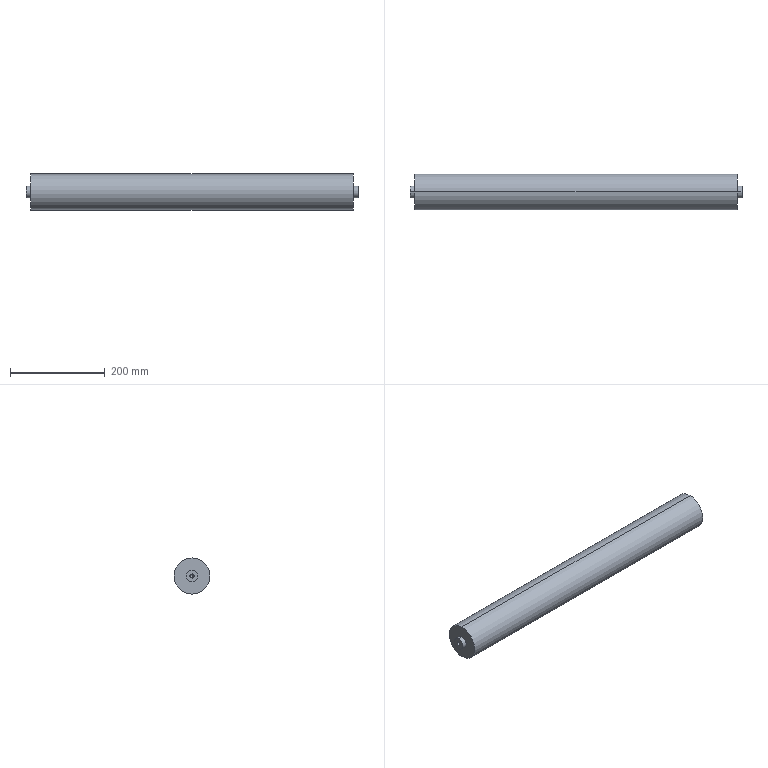Part | STEP file | φ76-700 | 1 solid | 18 faces | box 700 x 76 x 76 mm | volume 3091733 mm3 | cylinder 10 | cone 4 | plane 4 | commonest cylinder face diameters 8.5 x4 25 x4 76 x2
STEP:
#1=CARTESIAN_POINT('',(0.,0.,0.));
#2=DIRECTION('',(0.,0.,1.));
#3=DIRECTION('',(1.,0.,0.));
#4=AXIS2_PLACEMENT_3D('',#1,#2,#3);
#5=CARTESIAN_POINT('',(675.5,0.,-4.25));
#6=VERTEX_POINT('',#5);
#7=CARTESIAN_POINT('',(700.,0.,-4.25));
#8=VERTEX_POINT('',#7);
#9=CARTESIAN_POINT('',(700.,0.,-4.25));
#10=DIRECTION('',(1.,0.,0.));
#11=VECTOR('',#10,1.);
#12=LINE('',#9,#11);
#13=CARTESIAN_POINT('',(700.,0.,0.));
#14=DIRECTION('',(1.,0.,0.));
#15=DIRECTION('',(0.,0.,-1.));
#16=AXIS2_PLACEMENT_3D('',#13,#14,#15);
#17=CYLINDRICAL_SURFACE('',#16,4.25);
#18=CARTESIAN_POINT('',(6.283,0.));
#19=DIRECTION('',(0.,1.));
#20=VECTOR('',#19,1.);
#21=LINE('',#18,#20);
#22=(GEOMETRIC_REPRESENTATION_CONTEXT(2)PARAMETRIC_REPRESENTATION_CONTEXT()REPRESENTATION_CONTEXT('',''));
#23=DEFINITIONAL_REPRESENTATION('',(#21),#22);
#24=PCURVE('',#17,#23);
#25=CARTESIAN_POINT('',(700.,0.,0.));
#26=DIRECTION('',(1.,0.,0.));
#27=DIRECTION('',(0.,0.,-1.));
#28=AXIS2_PLACEMENT_3D('',#25,#26,#27);
#29=CYLINDRICAL_SURFACE('',#28,4.25);
#30=CARTESIAN_POINT('',(0.,0.));
#31=DIRECTION('',(0.,1.));
#32=VECTOR('',#31,1.);
#33=LINE('',#30,#32);
#34=(GEOMETRIC_REPRESENTATION_CONTEXT(2)PARAMETRIC_REPRESENTATION_CONTEXT()REPRESENTATION_CONTEXT('',''));
#35=DEFINITIONAL_REPRESENTATION('',(#33),#34);
#36=PCURVE('',#29,#35);
#37=SURFACE_CURVE('',#12,(#24,#36),.PCURVE_S1.);
#38=EDGE_CURVE('',#6,#8,#37,.T.);
#39=ORIENTED_EDGE('',*,*,#38,.T.);
#40=CARTESIAN_POINT('',(700.,0.,4.25));
#41=VERTEX_POINT('',#40);
#42=CARTESIAN_POINT('',(700.,0.,0.));
#43=DIRECTION('',(1.,0.,0.));
#44=DIRECTION('',(0.,0.,-1.));
#45=AXIS2_PLACEMENT_3D('',#42,#43,#44);
#46=CIRCLE('',#45,4.25);
#47=CARTESIAN_POINT('',(0.,0.));
#48=DIRECTION('',(1.,0.));
#49=VECTOR('',#48,1.);
#50=LINE('',#47,#49);
#51=(GEOMETRIC_REPRESENTATION_CONTEXT(2)PARAMETRIC_REPRESENTATION_CONTEXT()REPRESENTATION_CONTEXT('',''));
#52=DEFINITIONAL_REPRESENTATION('',(#50),#51);
#53=PCURVE('',#17,#52);
#54=CARTESIAN_POINT('',(700.,0.,0.));
#55=DIRECTION('',(-1.,0.,0.));
#56=DIRECTION('',(0.,0.,1.));
#57=AXIS2_PLACEMENT_3D('',#54,#55,#56);
#58=PLANE('',#57);
#59=CARTESIAN_POINT('',(-4.25,0.));
#60=CARTESIAN_POINT('',(-4.25,7.361));
#61=CARTESIAN_POINT('',(2.125,3.681));
#62=CARTESIAN_POINT('',(8.5,0.));
#63=CARTESIAN_POINT('',(2.125,-3.681));
#64=CARTESIAN_POINT('',(-4.25,-7.361));
#65=CARTESIAN_POINT('',(-4.25,0.));
#66=(BOUNDED_CURVE()B_SPLINE_CURVE(2,(#59,#60,#61,#62,#63,#64,#65),.UNSPECIFIED.,.T.,.F.)B_SPLINE_CURVE_WITH_KNOTS((1,2,2,2,2,1),(-2.094,0.,2.094,4.189,6.283,8.378),.UNSPECIFIED.)CURVE()GEOMETRIC_REPRESENTATION_ITEM()RATIONAL_B_SPLINE_CURVE((1.,0.5,1.,0.5,1.,0.5,1.))REPRESENTATION_ITEM(''));
#67=(GEOMETRIC_REPRESENTATION_CONTEXT(2)PARAMETRIC_REPRESENTATION_CONTEXT()REPRESENTATION_CONTEXT('',''));
#68=DEFINITIONAL_REPRESENTATION('',(#66),#67);
#69=PCURVE('',#58,#68);
#70=SURFACE_CURVE('',#46,(#53,#69),.PCURVE_S1.);
#71=EDGE_CURVE('',#41,#8,#70,.T.);
#72=ORIENTED_EDGE('',*,*,#71,.F.);
#73=CARTESIAN_POINT('',(675.5,0.,4.25));
#74=VERTEX_POINT('',#73);
#75=CARTESIAN_POINT('',(700.,0.,4.25));
#76=DIRECTION('',(1.,0.,0.));
#77=VECTOR('',#76,1.);
#78=LINE('',#75,#77);
#79=CARTESIAN_POINT('',(3.142,0.));
#80=DIRECTION('',(0.,1.));
#81=VECTOR('',#80,1.);
#82=LINE('',#79,#81);
#83=(GEOMETRIC_REPRESENTATION_CONTEXT(2)PARAMETRIC_REPRESENTATION_CONTEXT()REPRESENTATION_CONTEXT('',''));
#84=DEFINITIONAL_REPRESENTATION('',(#82),#83);
#85=PCURVE('',#17,#84);
#86=CARTESIAN_POINT('',(3.142,0.));
#87=DIRECTION('',(0.,1.));
#88=VECTOR('',#87,1.);
#89=LINE('',#86,#88);
#90=(GEOMETRIC_REPRESENTATION_CONTEXT(2)PARAMETRIC_REPRESENTATION_CONTEXT()REPRESENTATION_CONTEXT('',''));
#91=DEFINITIONAL_REPRESENTATION('',(#89),#90);
#92=PCURVE('',#29,#91);
#93=SURFACE_CURVE('',#78,(#85,#92),.PCURVE_S1.);
#94=EDGE_CURVE('',#74,#41,#93,.T.);
#95=ORIENTED_EDGE('',*,*,#94,.F.);
#96=CARTESIAN_POINT('',(675.5,0.,0.));
#97=DIRECTION('',(1.,0.,0.));
#98=DIRECTION('',(0.,0.,-1.));
#99=AXIS2_PLACEMENT_3D('',#96,#97,#98);
#100=CIRCLE('',#99,4.25);
#101=CARTESIAN_POINT('',(0.,-24.5));
#102=DIRECTION('',(1.,0.));
#103=VECTOR('',#102,1.);
#104=LINE('',#101,#103);
#105=(GEOMETRIC_REPRESENTATION_CONTEXT(2)PARAMETRIC_REPRESENTATION_CONTEXT()REPRESENTATION_CONTEXT('',''));
#106=DEFINITIONAL_REPRESENTATION('',(#104),#105);
#107=PCURVE('',#17,#106);
#108=CARTESIAN_POINT('',(675.5,0.,0.));
#109=DIRECTION('',(1.,0.,0.));
#110=DIRECTION('',(0.,0.,-1.));
#111=AXIS2_PLACEMENT_3D('',#108,#109,#110);
#112=CONICAL_SURFACE('',#111,4.25,1.03);
#113=CARTESIAN_POINT('',(0.,0.));
#114=DIRECTION('',(1.,0.));
#115=VECTOR('',#114,1.);
#116=LINE('',#113,#115);
#117=(GEOMETRIC_REPRESENTATION_CONTEXT(2)PARAMETRIC_REPRESENTATION_CONTEXT()REPRESENTATION_CONTEXT('',''));
#118=DEFINITIONAL_REPRESENTATION('',(#116),#117);
#119=PCURVE('',#112,#118);
#120=SURFACE_CURVE('',#100,(#107,#119),.PCURVE_S1.);
#121=EDGE_CURVE('',#74,#6,#120,.T.);
#122=ORIENTED_EDGE('',*,*,#121,.T.);
#123=EDGE_LOOP('',(#39,#72,#95,#122));
#124=FACE_BOUND('',#123,.F.);
#125=ADVANCED_FACE('',(#124),#17,.F.);
#126=ORIENTED_EDGE('',*,*,#121,.F.);
#127=CARTESIAN_POINT('',(672.946,0.,0.));
#128=VERTEX_POINT('',#127);
#129=CARTESIAN_POINT('',(675.5,0.,4.25));
#130=DIRECTION('',(0.515,0.,0.8572));
#131=VECTOR('',#130,1.);
#132=LINE('',#129,#131);
#133=CARTESIAN_POINT('',(3.142,0.));
#134=DIRECTION('',(0.,1.));
#135=VECTOR('',#134,1.);
#136=LINE('',#133,#135);
#137=(GEOMETRIC_REPRESENTATION_CONTEXT(2)PARAMETRIC_REPRESENTATION_CONTEXT()REPRESENTATION_CONTEXT('',''));
#138=DEFINITIONAL_REPRESENTATION('',(#136),#137);
#139=PCURVE('',#112,#138);
#140=CARTESIAN_POINT('',(675.5,0.,0.));
#141=DIRECTION('',(1.,0.,0.));
#142=DIRECTION('',(0.,0.,-1.));
#143=AXIS2_PLACEMENT_3D('',#140,#141,#142);
#144=CONICAL_SURFACE('',#143,4.25,1.03);
#145=CARTESIAN_POINT('',(3.142,0.));
#146=DIRECTION('',(0.,1.));
#147=VECTOR('',#146,1.);
#148=LINE('',#145,#147);
#149=(GEOMETRIC_REPRESENTATION_CONTEXT(2)PARAMETRIC_REPRESENTATION_CONTEXT()REPRESENTATION_CONTEXT('',''));
#150=DEFINITIONAL_REPRESENTATION('',(#148),#149);
#151=PCURVE('',#144,#150);
#152=SURFACE_CURVE('',#132,(#139,#151),.PCURVE_S1.);
#153=EDGE_CURVE('',#128,#74,#152,.T.);
#154=ORIENTED_EDGE('',*,*,#153,.F.);
#155=CARTESIAN_POINT('',(675.5,0.,-4.25));
#156=DIRECTION('',(0.515,0.,-0.8572));
#157=VECTOR('',#156,1.);
#158=LINE('',#155,#157);
#159=CARTESIAN_POINT('',(6.283,0.));
#160=DIRECTION('',(0.,1.));
#161=VECTOR('',#160,1.);
#162=LINE('',#159,#161);
#163=(GEOMETRIC_REPRESENTATION_CONTEXT(2)PARAMETRIC_REPRESENTATION_CONTEXT()REPRESENTATION_CONTEXT('',''));
#164=DEFINITIONAL_REPRESENTATION('',(#162),#163);
#165=PCURVE('',#112,#164);
#166=CARTESIAN_POINT('',(0.,0.));
#167=DIRECTION('',(0.,1.));
#168=VECTOR('',#167,1.);
#169=LINE('',#166,#168);
#170=(GEOMETRIC_REPRESENTATION_CONTEXT(2)PARAMETRIC_REPRESENTATION_CONTEXT()REPRESENTATION_CONTEXT('',''));
#171=DEFINITIONAL_REPRESENTATION('',(#169),#170);
#172=PCURVE('',#144,#171);
#173=SURFACE_CURVE('',#158,(#165,#172),.PCURVE_S1.);
#174=EDGE_CURVE('',#128,#6,#173,.T.);
#175=ORIENTED_EDGE('',*,*,#174,.T.);
#176=EDGE_LOOP('',(#126,#154,#175));
#177=FACE_BOUND('',#176,.F.);
#178=ADVANCED_FACE('',(#177),#112,.F.);
#179=CARTESIAN_POINT('',(24.5,0.,4.25));
#180=VERTEX_POINT('',#179);
#181=CARTESIAN_POINT('',(0.,0.,4.25));
#182=VERTEX_POINT('',#181);
#183=CARTESIAN_POINT('',(0.,0.,4.25));
#184=DIRECTION('',(-1.,0.,0.));
#185=VECTOR('',#184,1.);
#186=LINE('',#183,#185);
#187=CARTESIAN_POINT('',(0.,0.,0.));
#188=DIRECTION('',(-1.,0.,0.));
#189=DIRECTION('',(0.,0.,1.));
#190=AXIS2_PLACEMENT_3D('',#187,#188,#189);
#191=CYLINDRICAL_SURFACE('',#190,4.25);
#192=CARTESIAN_POINT('',(6.283,0.));
#193=DIRECTION('',(0.,1.));
#194=VECTOR('',#193,1.);
#195=LINE('',#192,#194);
#196=(GEOMETRIC_REPRESENTATION_CONTEXT(2)PARAMETRIC_REPRESENTATION_CONTEXT()REPRESENTATION_CONTEXT('',''));
#197=DEFINITIONAL_REPRESENTATION('',(#195),#196);
#198=PCURVE('',#191,#197);
#199=CARTESIAN_POINT('',(0.,0.,0.));
#200=DIRECTION('',(-1.,0.,0.));
#201=DIRECTION('',(0.,0.,1.));
#202=AXIS2_PLACEMENT_3D('',#199,#200,#201);
#203=CYLINDRICAL_SURFACE('',#202,4.25);
#204=CARTESIAN_POINT('',(0.,0.));
#205=DIRECTION('',(0.,1.));
#206=VECTOR('',#205,1.);
#207=LINE('',#204,#206);
#208=(GEOMETRIC_REPRESENTATION_CONTEXT(2)PARAMETRIC_REPRESENTATION_CONTEXT()REPRESENTATION_CONTEXT('',''));
#209=DEFINITIONAL_REPRESENTATION('',(#207),#208);
#210=PCURVE('',#203,#209);
#211=SURFACE_CURVE('',#186,(#198,#210),.PCURVE_S1.);
#212=EDGE_CURVE('',#180,#182,#211,.T.);
#213=ORIENTED_EDGE('',*,*,#212,.T.);
#214=CARTESIAN_POINT('',(0.,0.,-4.25));
#215=VERTEX_POINT('',#214);
#216=CARTESIAN_POINT('',(0.,0.,0.));
#217=DIRECTION('',(-1.,0.,0.));
#218=DIRECTION('',(0.,0.,1.));
#219=AXIS2_PLACEMENT_3D('',#216,#217,#218);
#220=CIRCLE('',#219,4.25);
#221=CARTESIAN_POINT('',(0.,0.));
#222=DIRECTION('',(1.,0.));
#223=VECTOR('',#222,1.);
#224=LINE('',#221,#223);
#225=(GEOMETRIC_REPRESENTATION_CONTEXT(2)PARAMETRIC_REPRESENTATION_CONTEXT()REPRESENTATION_CONTEXT('',''));
#226=DEFINITIONAL_REPRESENTATION('',(#224),#225);
#227=PCURVE('',#191,#226);
#228=CARTESIAN_POINT('',(0.,0.,0.));
#229=DIRECTION('',(1.,0.,0.));
#230=DIRECTION('',(0.,0.,-1.));
#231=AXIS2_PLACEMENT_3D('',#228,#229,#230);
#232=PLANE('',#231);
#233=CARTESIAN_POINT('',(-4.25,0.));
#234=CARTESIAN_POINT('',(-4.25,7.361));
#235=CARTESIAN_POINT('',(2.125,3.681));
#236=CARTESIAN_POINT('',(8.5,0.));
#237=CARTESIAN_POINT('',(2.125,-3.681));
#238=CARTESIAN_POINT('',(-4.25,-7.361));
#239=CARTESIAN_POINT('',(-4.25,0.));
#240=(BOUNDED_CURVE()B_SPLINE_CURVE(2,(#233,#234,#235,#236,#237,#238,#239),.UNSPECIFIED.,.T.,.F.)B_SPLINE_CURVE_WITH_KNOTS((1,2,2,2,2,1),(-2.094,0.,2.094,4.189,6.283,8.378),.UNSPECIFIED.)CURVE()GEOMETRIC_REPRESENTATION_ITEM()RATIONAL_B_SPLINE_CURVE((1.,0.5,1.,0.5,1.,0.5,1.))REPRESENTATION_ITEM(''));
#241=(GEOMETRIC_REPRESENTATION_CONTEXT(2)PARAMETRIC_REPRESENTATION_CONTEXT()REPRESENTATION_CONTEXT('',''));
#242=DEFINITIONAL_REPRESENTATION('',(#240),#241);
#243=PCURVE('',#232,#242);
#244=SURFACE_CURVE('',#220,(#227,#243),.PCURVE_S1.);
#245=EDGE_CURVE('',#215,#182,#244,.T.);
#246=ORIENTED_EDGE('',*,*,#245,.F.);
#247=CARTESIAN_POINT('',(24.5,0.,-4.25));
#248=VERTEX_POINT('',#247);
#249=CARTESIAN_POINT('',(0.,0.,-4.25));
#250=DIRECTION('',(-1.,0.,0.));
#251=VECTOR('',#250,1.);
#252=LINE('',#249,#251);
#253=CARTESIAN_POINT('',(3.142,0.));
#254=DIRECTION('',(0.,1.));
#255=VECTOR('',#254,1.);
#256=LINE('',#253,#255);
#257=(GEOMETRIC_REPRESENTATION_CONTEXT(2)PARAMETRIC_REPRESENTATION_CONTEXT()REPRESENTATION_CONTEXT('',''));
#258=DEFINITIONAL_REPRESENTATION('',(#256),#257);
#259=PCURVE('',#191,#258);
#260=CARTESIAN_POINT('',(3.142,0.));
#261=DIRECTION('',(0.,1.));
#262=VECTOR('',#261,1.);
#263=LINE('',#260,#262);
#264=(GEOMETRIC_REPRESENTATION_CONTEXT(2)PARAMETRIC_REPRESENTATION_CONTEXT()REPRESENTATION_CONTEXT('',''));
#265=DEFINITIONAL_REPRESENTATION('',(#263),#264);
#266=PCURVE('',#203,#265);
#267=SURFACE_CURVE('',#252,(#259,#266),.PCURVE_S1.);
#268=EDGE_CURVE('',#248,#215,#267,.T.);
#269=ORIENTED_EDGE('',*,*,#268,.F.);
#270=CARTESIAN_POINT('',(24.5,0.,0.));
#271=DIRECTION('',(-1.,0.,0.));
#272=DIRECTION('',(0.,0.,1.));
#273=AXIS2_PLACEMENT_3D('',#270,#271,#272);
#274=CIRCLE('',#273,4.25);
#275=CARTESIAN_POINT('',(0.,-24.5));
#276=DIRECTION('',(1.,0.));
#277=VECTOR('',#276,1.);
#278=LINE('',#275,#277);
#279=(GEOMETRIC_REPRESENTATION_CONTEXT(2)PARAMETRIC_REPRESENTATION_CONTEXT()REPRESENTATION_CONTEXT('',''));
#280=DEFINITIONAL_REPRESENTATION('',(#278),#279);
#281=PCURVE('',#191,#280);
#282=CARTESIAN_POINT('',(24.5,0.,0.));
#283=DIRECTION('',(-1.,0.,0.));
#284=DIRECTION('',(0.,0.,1.));
#285=AXIS2_PLACEMENT_3D('',#282,#283,#284);
#286=CONICAL_SURFACE('',#285,4.25,1.03);
#287=CARTESIAN_POINT('',(0.,0.));
#288=DIRECTION('',(1.,0.));
#289=VECTOR('',#288,1.);
#290=LINE('',#287,#289);
#291=(GEOMETRIC_REPRESENTATION_CONTEXT(2)PARAMETRIC_REPRESENTATION_CONTEXT()REPRESENTATION_CONTEXT('',''));
#292=DEFINITIONAL_REPRESENTATION('',(#290),#291);
#293=PCURVE('',#286,#292);
#294=SURFACE_CURVE('',#274,(#281,#293),.PCURVE_S1.);
#295=EDGE_CURVE('',#248,#180,#294,.T.);
#296=ORIENTED_EDGE('',*,*,#295,.T.);
#297=EDGE_LOOP('',(#213,#246,#269,#296));
#298=FACE_BOUND('',#297,.F.);
#299=ADVANCED_FACE('',(#298),#191,.F.);
#300=ORIENTED_EDGE('',*,*,#295,.F.);
#301=CARTESIAN_POINT('',(27.054,0.,0.));
#302=VERTEX_POINT('',#301);
#303=CARTESIAN_POINT('',(24.5,0.,-4.25));
#304=DIRECTION('',(-0.515,0.,-0.8572));
#305=VECTOR('',#304,1.);
#306=LINE('',#303,#305);
#307=CARTESIAN_POINT('',(3.142,0.));
#308=DIRECTION('',(0.,1.));
#309=VECTOR('',#308,1.);
#310=LINE('',#307,#309);
#311=(GEOMETRIC_REPRESENTATION_CONTEXT(2)PARAMETRIC_REPRESENTATION_CONTEXT()REPRESENTATION_CONTEXT('',''));
#312=DEFINITIONAL_REPRESENTATION('',(#310),#311);
#313=PCURVE('',#286,#312);
#314=CARTESIAN_POINT('',(24.5,0.,0.));
#315=DIRECTION('',(-1.,0.,0.));
#316=DIRECTION('',(0.,0.,1.));
#317=AXIS2_PLACEMENT_3D('',#314,#315,#316);
#318=CONICAL_SURFACE('',#317,4.25,1.03);
#319=CARTESIAN_POINT('',(3.142,0.));
#320=DIRECTION('',(0.,1.));
#321=VECTOR('',#320,1.);
#322=LINE('',#319,#321);
#323=(GEOMETRIC_REPRESENTATION_CONTEXT(2)PARAMETRIC_REPRESENTATION_CONTEXT()REPRESENTATION_CONTEXT('',''));
#324=DEFINITIONAL_REPRESENTATION('',(#322),#323);
#325=PCURVE('',#318,#324);
#326=SURFACE_CURVE('',#306,(#313,#325),.PCURVE_S1.);
#327=EDGE_CURVE('',#302,#248,#326,.T.);
#328=ORIENTED_EDGE('',*,*,#327,.F.);
#329=CARTESIAN_POINT('',(24.5,0.,4.25));
#330=DIRECTION('',(-0.515,0.,0.8572));
#331=VECTOR('',#330,1.);
#332=LINE('',#329,#331);
#333=CARTESIAN_POINT('',(6.283,0.));
#334=DIRECTION('',(0.,1.));
#335=VECTOR('',#334,1.);
#336=LINE('',#333,#335);
#337=(GEOMETRIC_REPRESENTATION_CONTEXT(2)PARAMETRIC_REPRESENTATION_CONTEXT()REPRESENTATION_CONTEXT('',''));
#338=DEFINITIONAL_REPRESENTATION('',(#336),#337);
#339=PCURVE('',#286,#338);
#340=CARTESIAN_POINT('',(0.,0.));
#341=DIRECTION('',(0.,1.));
#342=VECTOR('',#341,1.);
#343=LINE('',#340,#342);
#344=(GEOMETRIC_REPRESENTATION_CONTEXT(2)PARAMETRIC_REPRESENTATION_CONTEXT()REPRESENTATION_CONTEXT('',''));
#345=DEFINITIONAL_REPRESENTATION('',(#343),#344);
#346=PCURVE('',#318,#345);
#347=SURFACE_CURVE('',#332,(#339,#346),.PCURVE_S1.);
#348=EDGE_CURVE('',#302,#180,#347,.T.);
#349=ORIENTED_EDGE('',*,*,#348,.T.);
#350=EDGE_LOOP('',(#300,#328,#349));
#351=FACE_BOUND('',#350,.F.);
#352=ADVANCED_FACE('',(#351),#286,.F.);
#353=CARTESIAN_POINT('',(10.,0.,12.5));
#354=VERTEX_POINT('',#353);
#355=CARTESIAN_POINT('',(10.,0.,-12.5));
#356=VERTEX_POINT('',#355);
#357=CARTESIAN_POINT('',(10.,0.,0.));
#358=DIRECTION('',(-1.,0.,0.));
#359=DIRECTION('',(0.,0.,1.));
#360=AXIS2_PLACEMENT_3D('',#357,#358,#359);
#361=CIRCLE('',#360,12.5);
#362=CARTESIAN_POINT('',(0.,0.,0.));
#363=DIRECTION('',(-1.,0.,0.));
#364=DIRECTION('',(0.,0.,1.));
#365=AXIS2_PLACEMENT_3D('',#362,#363,#364);
#366=CYLINDRICAL_SURFACE('',#365,12.5);
#367=CARTESIAN_POINT('',(0.,-10.));
#368=DIRECTION('',(1.,0.));
#369=VECTOR('',#368,1.);
#370=LINE('',#367,#369);
#371=(GEOMETRIC_REPRESENTATION_CONTEXT(2)PARAMETRIC_REPRESENTATION_CONTEXT()REPRESENTATION_CONTEXT('',''));
#372=DEFINITIONAL_REPRESENTATION('',(#370),#371);
#373=PCURVE('',#366,#372);
#374=CARTESIAN_POINT('',(10.,38.,0.));
#375=DIRECTION('',(1.,0.,0.));
#376=DIRECTION('',(0.,0.,-1.));
#377=AXIS2_PLACEMENT_3D('',#374,#375,#376);
#378=PLANE('',#377);
#379=CARTESIAN_POINT('',(-12.5,-38.));
#380=CARTESIAN_POINT('',(-12.5,-16.349));
#381=CARTESIAN_POINT('',(6.25,-27.175));
#382=CARTESIAN_POINT('',(25.,-38.));
#383=CARTESIAN_POINT('',(6.25,-48.825));
#384=CARTESIAN_POINT('',(-12.5,-59.651));
#385=CARTESIAN_POINT('',(-12.5,-38.));
#386=(BOUNDED_CURVE()B_SPLINE_CURVE(2,(#379,#380,#381,#382,#383,#384,#385),.UNSPECIFIED.,.T.,.F.)B_SPLINE_CURVE_WITH_KNOTS((1,2,2,2,2,1),(-2.094,0.,2.094,4.189,6.283,8.378),.UNSPECIFIED.)CURVE()GEOMETRIC_REPRESENTATION_ITEM()RATIONAL_B_SPLINE_CURVE((1.,0.5,1.,0.5,1.,0.5,1.))REPRESENTATION_ITEM(''));
#387=(GEOMETRIC_REPRESENTATION_CONTEXT(2)PARAMETRIC_REPRESENTATION_CONTEXT()REPRESENTATION_CONTEXT('',''));
#388=DEFINITIONAL_REPRESENTATION('',(#386),#387);
#389=PCURVE('',#378,#388);
#390=SURFACE_CURVE('',#361,(#373,#389),.PCURVE_S1.);
#391=EDGE_CURVE('',#354,#356,#390,.T.);
#392=ORIENTED_EDGE('',*,*,#391,.T.);
#393=CARTESIAN_POINT('',(0.,0.,-12.5));
#394=VERTEX_POINT('',#393);
#395=CARTESIAN_POINT('',(0.,0.,-12.5));
#396=DIRECTION('',(-1.,0.,0.));
#397=VECTOR('',#396,1.);
#398=LINE('',#395,#397);
#399=CARTESIAN_POINT('',(3.142,0.));
#400=DIRECTION('',(0.,1.));
#401=VECTOR('',#400,1.);
#402=LINE('',#399,#401);
#403=(GEOMETRIC_REPRESENTATION_CONTEXT(2)PARAMETRIC_REPRESENTATION_CONTEXT()REPRESENTATION_CONTEXT('',''));
#404=DEFINITIONAL_REPRESENTATION('',(#402),#403);
#405=PCURVE('',#366,#404);
#406=CARTESIAN_POINT('',(0.,0.,0.));
#407=DIRECTION('',(-1.,0.,0.));
#408=DIRECTION('',(0.,0.,1.));
#409=AXIS2_PLACEMENT_3D('',#406,#407,#408);
#410=CYLINDRICAL_SURFACE('',#409,12.5);
#411=CARTESIAN_POINT('',(3.142,0.));
#412=DIRECTION('',(0.,1.));
#413=VECTOR('',#412,1.);
#414=LINE('',#411,#413);
#415=(GEOMETRIC_REPRESENTATION_CONTEXT(2)PARAMETRIC_REPRESENTATION_CONTEXT()REPRESENTATION_CONTEXT('',''));
#416=DEFINITIONAL_REPRESENTATION('',(#414),#415);
#417=PCURVE('',#410,#416);
#418=SURFACE_CURVE('',#398,(#405,#417),.PCURVE_S1.);
#419=EDGE_CURVE('',#356,#394,#418,.T.);
#420=ORIENTED_EDGE('',*,*,#419,.T.);
#421=CARTESIAN_POINT('',(0.,0.,12.5));
#422=VERTEX_POINT('',#421);
#423=CARTESIAN_POINT('',(0.,0.,0.));
#424=DIRECTION('',(-1.,0.,0.));
#425=DIRECTION('',(0.,0.,1.));
#426=AXIS2_PLACEMENT_3D('',#423,#424,#425);
#427=CIRCLE('',#426,12.5);
#428=CARTESIAN_POINT('',(0.,0.));
#429=DIRECTION('',(1.,0.));
#430=VECTOR('',#429,1.);
#431=LINE('',#428,#430);
#432=(GEOMETRIC_REPRESENTATION_CONTEXT(2)PARAMETRIC_REPRESENTATION_CONTEXT()REPRESENTATION_CONTEXT('',''));
#433=DEFINITIONAL_REPRESENTATION('',(#431),#432);
#434=PCURVE('',#366,#433);
#435=CARTESIAN_POINT('',(-12.5,0.));
#436=CARTESIAN_POINT('',(-12.5,21.651));
#437=CARTESIAN_POINT('',(6.25,10.825));
#438=CARTESIAN_POINT('',(25.,0.));
#439=CARTESIAN_POINT('',(6.25,-10.825));
#440=CARTESIAN_POINT('',(-12.5,-21.651));
#441=CARTESIAN_POINT('',(-12.5,0.));
#442=(BOUNDED_CURVE()B_SPLINE_CURVE(2,(#435,#436,#437,#438,#439,#440,#441),.UNSPECIFIED.,.T.,.F.)B_SPLINE_CURVE_WITH_KNOTS((1,2,2,2,2,1),(-2.094,0.,2.094,4.189,6.283,8.378),.UNSPECIFIED.)CURVE()GEOMETRIC_REPRESENTATION_ITEM()RATIONAL_B_SPLINE_CURVE((1.,0.5,1.,0.5,1.,0.5,1.))REPRESENTATION_ITEM(''));
#443=(GEOMETRIC_REPRESENTATION_CONTEXT(2)PARAMETRIC_REPRESENTATION_CONTEXT()REPRESENTATION_CONTEXT('',''));
#444=DEFINITIONAL_REPRESENTATION('',(#442),#443);
#445=PCURVE('',#232,#444);
#446=SURFACE_CURVE('',#427,(#434,#445),.PCURVE_S1.);
#447=EDGE_CURVE('',#422,#394,#446,.T.);
#448=ORIENTED_EDGE('',*,*,#447,.F.);
#449=CARTESIAN_POINT('',(0.,0.,12.5));
#450=DIRECTION('',(-1.,0.,0.));
#451=VECTOR('',#450,1.);
#452=LINE('',#449,#451);
#453=CARTESIAN_POINT('',(0.,0.));
#454=DIRECTION('',(0.,1.));
#455=VECTOR('',#454,1.);
#456=LINE('',#453,#455);
#457=(GEOMETRIC_REPRESENTATION_CONTEXT(2)PARAMETRIC_REPRESENTATION_CONTEXT()REPRESENTATION_CONTEXT('',''));
#458=DEFINITIONAL_REPRESENTATION('',(#456),#457);
#459=PCURVE('',#366,#458);
#460=CARTESIAN_POINT('',(6.283,0.));
#461=DIRECTION('',(0.,1.));
#462=VECTOR('',#461,1.);
#463=LINE('',#460,#462);
#464=(GEOMETRIC_REPRESENTATION_CONTEXT(2)PARAMETRIC_REPRESENTATION_CONTEXT()REPRESENTATION_CONTEXT('',''));
#465=DEFINITIONAL_REPRESENTATION('',(#463),#464);
#466=PCURVE('',#410,#465);
#467=SURFACE_CURVE('',#452,(#459,#466),.PCURVE_S1.);
#468=EDGE_CURVE('',#354,#422,#467,.T.);
#469=ORIENTED_EDGE('',*,*,#468,.F.);
#470=EDGE_LOOP('',(#392,#420,#448,#469));
#471=FACE_BOUND('',#470,.T.);
#472=ADVANCED_FACE('',(#471),#366,.T.);
#473=CARTESIAN_POINT('',(690.,0.,38.));
#474=VERTEX_POINT('',#473);
#475=CARTESIAN_POINT('',(690.,0.,-38.));
#476=VERTEX_POINT('',#475);
#477=CARTESIAN_POINT('',(690.,0.,0.));
#478=DIRECTION('',(-1.,0.,0.));
#479=DIRECTION('',(0.,0.,1.));
#480=AXIS2_PLACEMENT_3D('',#477,#478,#479);
#481=CIRCLE('',#480,38.);
#482=CARTESIAN_POINT('',(0.,0.,0.));
#483=DIRECTION('',(-1.,0.,0.));
#484=DIRECTION('',(0.,0.,1.));
#485=AXIS2_PLACEMENT_3D('',#482,#483,#484);
#486=CYLINDRICAL_SURFACE('',#485,38.);
#487=CARTESIAN_POINT('',(0.,-690.));
#488=DIRECTION('',(1.,0.));
#489=VECTOR('',#488,1.);
#490=LINE('',#487,#489);
#491=(GEOMETRIC_REPRESENTATION_CONTEXT(2)PARAMETRIC_REPRESENTATION_CONTEXT()REPRESENTATION_CONTEXT('',''));
#492=DEFINITIONAL_REPRESENTATION('',(#490),#491);
#493=PCURVE('',#486,#492);
#494=CARTESIAN_POINT('',(690.,12.5,0.));
#495=DIRECTION('',(-1.,0.,0.));
#496=DIRECTION('',(0.,0.,1.));
#497=AXIS2_PLACEMENT_3D('',#494,#495,#496);
#498=PLANE('',#497);
#499=CARTESIAN_POINT('',(0.,-12.5));
#500=DIRECTION('',(1.,0.));
#501=AXIS2_PLACEMENT_2D('',#499,#500);
#502=CIRCLE('',#501,38.);
#503=(GEOMETRIC_REPRESENTATION_CONTEXT(2)PARAMETRIC_REPRESENTATION_CONTEXT()REPRESENTATION_CONTEXT('',''));
#504=DEFINITIONAL_REPRESENTATION('',(#502),#503);
#505=PCURVE('',#498,#504);
#506=SURFACE_CURVE('',#481,(#493,#505),.PCURVE_S1.);
#507=EDGE_CURVE('',#474,#476,#506,.T.);
#508=ORIENTED_EDGE('',*,*,#507,.T.);
#509=CARTESIAN_POINT('',(10.,0.,-38.));
#510=VERTEX_POINT('',#509);
#511=CARTESIAN_POINT('',(0.,0.,-38.));
#512=DIRECTION('',(-1.,0.,0.));
#513=VECTOR('',#512,1.);
#514=LINE('',#511,#513);
#515=CARTESIAN_POINT('',(3.142,0.));
#516=DIRECTION('',(0.,1.));
#517=VECTOR('',#516,1.);
#518=LINE('',#515,#517);
#519=(GEOMETRIC_REPRESENTATION_CONTEXT(2)PARAMETRIC_REPRESENTATION_CONTEXT()REPRESENTATION_CONTEXT('',''));
#520=DEFINITIONAL_REPRESENTATION('',(#518),#519);
#521=PCURVE('',#486,#520);
#522=CARTESIAN_POINT('',(0.,0.,0.));
#523=DIRECTION('',(-1.,0.,0.));
#524=DIRECTION('',(0.,0.,1.));
#525=AXIS2_PLACEMENT_3D('',#522,#523,#524);
#526=CYLINDRICAL_SURFACE('',#525,38.);
#527=CARTESIAN_POINT('',(3.142,0.));
#528=DIRECTION('',(0.,1.));
#529=VECTOR('',#528,1.);
#530=LINE('',#527,#529);
#531=(GEOMETRIC_REPRESENTATION_CONTEXT(2)PARAMETRIC_REPRESENTATION_CONTEXT()REPRESENTATION_CONTEXT('',''));
#532=DEFINITIONAL_REPRESENTATION('',(#530),#531);
#533=PCURVE('',#526,#532);
#534=SURFACE_CURVE('',#514,(#521,#533),.PCURVE_S1.);
#535=EDGE_CURVE('',#476,#510,#534,.T.);
#536=ORIENTED_EDGE('',*,*,#535,.T.);
#537=CARTESIAN_POINT('',(10.,0.,38.));
#538=VERTEX_POINT('',#537);
#539=CARTESIAN_POINT('',(10.,0.,0.));
#540=DIRECTION('',(-1.,0.,0.));
#541=DIRECTION('',(0.,0.,1.));
#542=AXIS2_PLACEMENT_3D('',#539,#540,#541);
#543=CIRCLE('',#542,38.);
#544=CARTESIAN_POINT('',(0.,-10.));
#545=DIRECTION('',(1.,0.));
#546=VECTOR('',#545,1.);
#547=LINE('',#544,#546);
#548=(GEOMETRIC_REPRESENTATION_CONTEXT(2)PARAMETRIC_REPRESENTATION_CONTEXT()REPRESENTATION_CONTEXT('',''));
#549=DEFINITIONAL_REPRESENTATION('',(#547),#548);
#550=PCURVE('',#486,#549);
#551=CARTESIAN_POINT('',(-38.,-38.));
#552=CARTESIAN_POINT('',(-38.,27.818));
#553=CARTESIAN_POINT('',(19.,-5.091));
#554=CARTESIAN_POINT('',(76.,-38.));
#555=CARTESIAN_POINT('',(19.,-70.909));
#556=CARTESIAN_POINT('',(-38.,-103.818));
#557=CARTESIAN_POINT('',(-38.,-38.));
#558=(BOUNDED_CURVE()B_SPLINE_CURVE(2,(#551,#552,#553,#554,#555,#556,#557),.UNSPECIFIED.,.T.,.F.)B_SPLINE_CURVE_WITH_KNOTS((1,2,2,2,2,1),(-2.094,0.,2.094,4.189,6.283,8.378),.UNSPECIFIED.)CURVE()GEOMETRIC_REPRESENTATION_ITEM()RATIONAL_B_SPLINE_CURVE((1.,0.5,1.,0.5,1.,0.5,1.))REPRESENTATION_ITEM(''));
#559=(GEOMETRIC_REPRESENTATION_CONTEXT(2)PARAMETRIC_REPRESENTATION_CONTEXT()REPRESENTATION_CONTEXT('',''));
#560=DEFINITIONAL_REPRESENTATION('',(#558),#559);
#561=PCURVE('',#378,#560);
#562=SURFACE_CURVE('',#543,(#550,#561),.PCURVE_S1.);
#563=EDGE_CURVE('',#538,#510,#562,.T.);
#564=ORIENTED_EDGE('',*,*,#563,.F.);
#565=CARTESIAN_POINT('',(0.,0.,38.));
#566=DIRECTION('',(-1.,0.,0.));
#567=VECTOR('',#566,1.);
#568=LINE('',#565,#567);
#569=CARTESIAN_POINT('',(0.,0.));
#570=DIRECTION('',(0.,1.));
#571=VECTOR('',#570,1.);
#572=LINE('',#569,#571);
#573=(GEOMETRIC_REPRESENTATION_CONTEXT(2)PARAMETRIC_REPRESENTATION_CONTEXT()REPRESENTATION_CONTEXT('',''));
#574=DEFINITIONAL_REPRESENTATION('',(#572),#573);
#575=PCURVE('',#486,#574);
#576=CARTESIAN_POINT('',(6.283,0.));
#577=DIRECTION('',(0.,1.));
#578=VECTOR('',#577,1.);
#579=LINE('',#576,#578);
#580=(GEOMETRIC_REPRESENTATION_CONTEXT(2)PARAMETRIC_REPRESENTATION_CONTEXT()REPRESENTATION_CONTEXT('',''));
#581=DEFINITIONAL_REPRESENTATION('',(#579),#580);
#582=PCURVE('',#526,#581);
#583=SURFACE_CURVE('',#568,(#575,#582),.PCURVE_S1.);
#584=EDGE_CURVE('',#474,#538,#583,.T.);
#585=ORIENTED_EDGE('',*,*,#584,.F.);
#586=EDGE_LOOP('',(#508,#536,#564,#585));
#587=FACE_BOUND('',#586,.T.);
#588=ADVANCED_FACE('',(#587),#486,.T.);
#589=CARTESIAN_POINT('',(700.,0.,12.5));
#590=VERTEX_POINT('',#589);
#591=CARTESIAN_POINT('',(700.,0.,-12.5));
#592=VERTEX_POINT('',#591);
#593=CARTESIAN_POINT('',(700.,0.,0.));
#594=DIRECTION('',(-1.,0.,0.));
#595=DIRECTION('',(0.,0.,1.));
#596=AXIS2_PLACEMENT_3D('',#593,#594,#595);
#597=CIRCLE('',#596,12.5);
#598=CARTESIAN_POINT('',(0.,0.,0.));
#599=DIRECTION('',(-1.,0.,0.));
#600=DIRECTION('',(0.,0.,1.));
#601=AXIS2_PLACEMENT_3D('',#598,#599,#600);
#602=CYLINDRICAL_SURFACE('',#601,12.5);
#603=CARTESIAN_POINT('',(0.,-700.));
#604=DIRECTION('',(1.,0.));
#605=VECTOR('',#604,1.);
#606=LINE('',#603,#605);
#607=(GEOMETRIC_REPRESENTATION_CONTEXT(2)PARAMETRIC_REPRESENTATION_CONTEXT()REPRESENTATION_CONTEXT('',''));
#608=DEFINITIONAL_REPRESENTATION('',(#606),#607);
#609=PCURVE('',#602,#608);
#610=CARTESIAN_POINT('',(0.,0.));
#611=DIRECTION('',(1.,0.));
#612=AXIS2_PLACEMENT_2D('',#610,#611);
#613=CIRCLE('',#612,12.5);
#614=(GEOMETRIC_REPRESENTATION_CONTEXT(2)PARAMETRIC_REPRESENTATION_CONTEXT()REPRESENTATION_CONTEXT('',''));
#615=DEFINITIONAL_REPRESENTATION('',(#613),#614);
#616=PCURVE('',#58,#615);
#617=SURFACE_CURVE('',#597,(#609,#616),.PCURVE_S1.);
#618=EDGE_CURVE('',#590,#592,#617,.T.);
#619=ORIENTED_EDGE('',*,*,#618,.T.);
#620=CARTESIAN_POINT('',(690.,0.,-12.5));
#621=VERTEX_POINT('',#620);
#622=CARTESIAN_POINT('',(0.,0.,-12.5));
#623=DIRECTION('',(-1.,0.,0.));
#624=VECTOR('',#623,1.);
#625=LINE('',#622,#624);
#626=CARTESIAN_POINT('',(3.142,0.));
#627=DIRECTION('',(0.,1.));
#628=VECTOR('',#627,1.);
#629=LINE('',#626,#628);
#630=(GEOMETRIC_REPRESENTATION_CONTEXT(2)PARAMETRIC_REPRESENTATION_CONTEXT()REPRESENTATION_CONTEXT('',''));
#631=DEFINITIONAL_REPRESENTATION('',(#629),#630);
#632=PCURVE('',#602,#631);
#633=CARTESIAN_POINT('',(0.,0.,0.));
#634=DIRECTION('',(-1.,0.,0.));
#635=DIRECTION('',(0.,0.,1.));
#636=AXIS2_PLACEMENT_3D('',#633,#634,#635);
#637=CYLINDRICAL_SURFACE('',#636,12.5);
#638=CARTESIAN_POINT('',(3.142,0.));
#639=DIRECTION('',(0.,1.));
#640=VECTOR('',#639,1.);
#641=LINE('',#638,#640);
#642=(GEOMETRIC_REPRESENTATION_CONTEXT(2)PARAMETRIC_REPRESENTATION_CONTEXT()REPRESENTATION_CONTEXT('',''));
#643=DEFINITIONAL_REPRESENTATION('',(#641),#642);
#644=PCURVE('',#637,#643);
#645=SURFACE_CURVE('',#625,(#632,#644),.PCURVE_S1.);
#646=EDGE_CURVE('',#592,#621,#645,.T.);
#647=ORIENTED_EDGE('',*,*,#646,.T.);
#648=CARTESIAN_POINT('',(690.,0.,12.5));
#649=VERTEX_POINT('',#648);
#650=CARTESIAN_POINT('',(690.,0.,0.));
#651=DIRECTION('',(-1.,0.,0.));
#652=DIRECTION('',(0.,0.,1.));
#653=AXIS2_PLACEMENT_3D('',#650,#651,#652);
#654=CIRCLE('',#653,12.5);
#655=CARTESIAN_POINT('',(0.,-690.));
#656=DIRECTION('',(1.,0.));
#657=VECTOR('',#656,1.);
#658=LINE('',#655,#657);
#659=(GEOMETRIC_REPRESENTATION_CONTEXT(2)PARAMETRIC_REPRESENTATION_CONTEXT()REPRESENTATION_CONTEXT('',''));
#660=DEFINITIONAL_REPRESENTATION('',(#658),#659);
#661=PCURVE('',#602,#660);
#662=CARTESIAN_POINT('',(0.,-12.5));
#663=DIRECTION('',(1.,0.));
#664=AXIS2_PLACEMENT_2D('',#662,#663);
#665=CIRCLE('',#664,12.5);
#666=(GEOMETRIC_REPRESENTATION_CONTEXT(2)PARAMETRIC_REPRESENTATION_CONTEXT()REPRESENTATION_CONTEXT('',''));
#667=DEFINITIONAL_REPRESENTATION('',(#665),#666);
#668=PCURVE('',#498,#667);
#669=SURFACE_CURVE('',#654,(#661,#668),.PCURVE_S1.);
#670=EDGE_CURVE('',#649,#621,#669,.T.);
#671=ORIENTED_EDGE('',*,*,#670,.F.);
#672=CARTESIAN_POINT('',(0.,0.,12.5));
#673=DIRECTION('',(-1.,0.,0.));
#674=VECTOR('',#673,1.);
#675=LINE('',#672,#674);
#676=CARTESIAN_POINT('',(0.,0.));
#677=DIRECTION('',(0.,1.));
#678=VECTOR('',#677,1.);
#679=LINE('',#676,#678);
#680=(GEOMETRIC_REPRESENTATION_CONTEXT(2)PARAMETRIC_REPRESENTATION_CONTEXT()REPRESENTATION_CONTEXT('',''));
#681=DEFINITIONAL_REPRESENTATION('',(#679),#680);
#682=PCURVE('',#602,#681);
#683=CARTESIAN_POINT('',(6.283,0.));
#684=DIRECTION('',(0.,1.));
#685=VECTOR('',#684,1.);
#686=LINE('',#683,#685);
#687=(GEOMETRIC_REPRESENTATION_CONTEXT(2)PARAMETRIC_REPRESENTATION_CONTEXT()REPRESENTATION_CONTEXT('',''));
#688=DEFINITIONAL_REPRESENTATION('',(#686),#687);
#689=PCURVE('',#637,#688);
#690=SURFACE_CURVE('',#675,(#682,#689),.PCURVE_S1.);
#691=EDGE_CURVE('',#590,#649,#690,.T.);
#692=ORIENTED_EDGE('',*,*,#691,.F.);
#693=EDGE_LOOP('',(#619,#647,#671,#692));
#694=FACE_BOUND('',#693,.T.);
#695=ADVANCED_FACE('',(#694),#602,.T.);
#696=CARTESIAN_POINT('',(0.,0.,0.));
#697=DIRECTION('',(-1.,0.,0.));
#698=DIRECTION('',(0.,0.,1.));
#699=AXIS2_PLACEMENT_3D('',#696,#697,#698);
#700=CIRCLE('',#699,4.25);
#701=CARTESIAN_POINT('',(-4.25,0.));
#702=CARTESIAN_POINT('',(-4.25,7.361));
#703=CARTESIAN_POINT('',(2.125,3.681));
#704=CARTESIAN_POINT('',(8.5,0.));
#705=CARTESIAN_POINT('',(2.125,-3.681));
#706=CARTESIAN_POINT('',(-4.25,-7.361));
#707=CARTESIAN_POINT('',(-4.25,0.));
#708=(BOUNDED_CURVE()B_SPLINE_CURVE(2,(#701,#702,#703,#704,#705,#706,#707),.UNSPECIFIED.,.T.,.F.)B_SPLINE_CURVE_WITH_KNOTS((1,2,2,2,2,1),(-2.094,0.,2.094,4.189,6.283,8.378),.UNSPECIFIED.)CURVE()GEOMETRIC_REPRESENTATION_ITEM()RATIONAL_B_SPLINE_CURVE((1.,0.5,1.,0.5,1.,0.5,1.))REPRESENTATION_ITEM(''));
#709=(GEOMETRIC_REPRESENTATION_CONTEXT(2)PARAMETRIC_REPRESENTATION_CONTEXT()REPRESENTATION_CONTEXT('',''));
#710=DEFINITIONAL_REPRESENTATION('',(#708),#709);
#711=PCURVE('',#232,#710);
#712=CARTESIAN_POINT('',(0.,0.));
#713=DIRECTION('',(1.,0.));
#714=VECTOR('',#713,1.);
#715=LINE('',#712,#714);
#716=(GEOMETRIC_REPRESENTATION_CONTEXT(2)PARAMETRIC_REPRESENTATION_CONTEXT()REPRESENTATION_CONTEXT('',''));
#717=DEFINITIONAL_REPRESENTATION('',(#715),#716);
#718=PCURVE('',#203,#717);
#719=SURFACE_CURVE('',#700,(#711,#718),.PCURVE_S1.);
#720=EDGE_CURVE('',#182,#215,#719,.T.);
#721=ORIENTED_EDGE('',*,*,#720,.F.);
#722=ORIENTED_EDGE('',*,*,#245,.F.);
#723=EDGE_LOOP('',(#721,#722));
#724=FACE_BOUND('',#723,.T.);
#725=ORIENTED_EDGE('',*,*,#447,.T.);
#726=CARTESIAN_POINT('',(0.,0.,0.));
#727=DIRECTION('',(-1.,0.,0.));
#728=DIRECTION('',(0.,0.,1.));
#729=AXIS2_PLACEMENT_3D('',#726,#727,#728);
#730=CIRCLE('',#729,12.5);
#731=CARTESIAN_POINT('',(-12.5,0.));
#732=CARTESIAN_POINT('',(-12.5,21.651));
#733=CARTESIAN_POINT('',(6.25,10.825));
#734=CARTESIAN_POINT('',(25.,0.));
#735=CARTESIAN_POINT('',(6.25,-10.825));
#736=CARTESIAN_POINT('',(-12.5,-21.651));
#737=CARTESIAN_POINT('',(-12.5,0.));
#738=(BOUNDED_CURVE()B_SPLINE_CURVE(2,(#731,#732,#733,#734,#735,#736,#737),.UNSPECIFIED.,.T.,.F.)B_SPLINE_CURVE_WITH_KNOTS((1,2,2,2,2,1),(-2.094,0.,2.094,4.189,6.283,8.378),.UNSPECIFIED.)CURVE()GEOMETRIC_REPRESENTATION_ITEM()RATIONAL_B_SPLINE_CURVE((1.,0.5,1.,0.5,1.,0.5,1.))REPRESENTATION_ITEM(''));
#739=(GEOMETRIC_REPRESENTATION_CONTEXT(2)PARAMETRIC_REPRESENTATION_CONTEXT()REPRESENTATION_CONTEXT('',''));
#740=DEFINITIONAL_REPRESENTATION('',(#738),#739);
#741=PCURVE('',#232,#740);
#742=CARTESIAN_POINT('',(0.,0.));
#743=DIRECTION('',(1.,0.));
#744=VECTOR('',#743,1.);
#745=LINE('',#742,#744);
#746=(GEOMETRIC_REPRESENTATION_CONTEXT(2)PARAMETRIC_REPRESENTATION_CONTEXT()REPRESENTATION_CONTEXT('',''));
#747=DEFINITIONAL_REPRESENTATION('',(#745),#746);
#748=PCURVE('',#410,#747);
#749=SURFACE_CURVE('',#730,(#741,#748),.PCURVE_S1.);
#750=EDGE_CURVE('',#394,#422,#749,.T.);
#751=ORIENTED_EDGE('',*,*,#750,.T.);
#752=EDGE_LOOP('',(#725,#751));
#753=FACE_BOUND('',#752,.T.);
#754=ADVANCED_FACE('',(#724,#753),#232,.F.);
#755=CARTESIAN_POINT('',(700.,0.,0.));
#756=DIRECTION('',(1.,0.,0.));
#757=DIRECTION('',(0.,0.,-1.));
#758=AXIS2_PLACEMENT_3D('',#755,#756,#757);
#759=CIRCLE('',#758,4.25);
#760=CARTESIAN_POINT('',(-4.25,0.));
#761=CARTESIAN_POINT('',(-4.25,7.361));
#762=CARTESIAN_POINT('',(2.125,3.681));
#763=CARTESIAN_POINT('',(8.5,0.));
#764=CARTESIAN_POINT('',(2.125,-3.681));
#765=CARTESIAN_POINT('',(-4.25,-7.361));
#766=CARTESIAN_POINT('',(-4.25,0.));
#767=(BOUNDED_CURVE()B_SPLINE_CURVE(2,(#760,#761,#762,#763,#764,#765,#766),.UNSPECIFIED.,.T.,.F.)B_SPLINE_CURVE_WITH_KNOTS((1,2,2,2,2,1),(-2.094,0.,2.094,4.189,6.283,8.378),.UNSPECIFIED.)CURVE()GEOMETRIC_REPRESENTATION_ITEM()RATIONAL_B_SPLINE_CURVE((1.,0.5,1.,0.5,1.,0.5,1.))REPRESENTATION_ITEM(''));
#768=(GEOMETRIC_REPRESENTATION_CONTEXT(2)PARAMETRIC_REPRESENTATION_CONTEXT()REPRESENTATION_CONTEXT('',''));
#769=DEFINITIONAL_REPRESENTATION('',(#767),#768);
#770=PCURVE('',#58,#769);
#771=CARTESIAN_POINT('',(0.,0.));
#772=DIRECTION('',(1.,0.));
#773=VECTOR('',#772,1.);
#774=LINE('',#771,#773);
#775=(GEOMETRIC_REPRESENTATION_CONTEXT(2)PARAMETRIC_REPRESENTATION_CONTEXT()REPRESENTATION_CONTEXT('',''));
#776=DEFINITIONAL_REPRESENTATION('',(#774),#775);
#777=PCURVE('',#29,#776);
#778=SURFACE_CURVE('',#759,(#770,#777),.PCURVE_S1.);
#779=EDGE_CURVE('',#8,#41,#778,.T.);
#780=ORIENTED_EDGE('',*,*,#779,.F.);
#781=ORIENTED_EDGE('',*,*,#71,.F.);
#782=EDGE_LOOP('',(#780,#781));
#783=FACE_BOUND('',#782,.T.);
#784=ORIENTED_EDGE('',*,*,#618,.F.);
#785=CARTESIAN_POINT('',(700.,0.,0.));
#786=DIRECTION('',(-1.,0.,0.));
#787=DIRECTION('',(0.,0.,1.));
#788=AXIS2_PLACEMENT_3D('',#785,#786,#787);
#789=CIRCLE('',#788,12.5);
#790=CARTESIAN_POINT('',(0.,0.));
#791=DIRECTION('',(1.,0.));
#792=AXIS2_PLACEMENT_2D('',#790,#791);
#793=CIRCLE('',#792,12.5);
#794=(GEOMETRIC_REPRESENTATION_CONTEXT(2)PARAMETRIC_REPRESENTATION_CONTEXT()REPRESENTATION_CONTEXT('',''));
#795=DEFINITIONAL_REPRESENTATION('',(#793),#794);
#796=PCURVE('',#58,#795);
#797=CARTESIAN_POINT('',(0.,-700.));
#798=DIRECTION('',(1.,0.));
#799=VECTOR('',#798,1.);
#800=LINE('',#797,#799);
#801=(GEOMETRIC_REPRESENTATION_CONTEXT(2)PARAMETRIC_REPRESENTATION_CONTEXT()REPRESENTATION_CONTEXT('',''));
#802=DEFINITIONAL_REPRESENTATION('',(#800),#801);
#803=PCURVE('',#637,#802);
#804=SURFACE_CURVE('',#789,(#796,#803),.PCURVE_S1.);
#805=EDGE_CURVE('',#592,#590,#804,.T.);
#806=ORIENTED_EDGE('',*,*,#805,.F.);
#807=EDGE_LOOP('',(#784,#806));
#808=FACE_BOUND('',#807,.T.);
#809=ADVANCED_FACE('',(#783,#808),#58,.F.);
#810=ORIENTED_EDGE('',*,*,#646,.F.);
#811=ORIENTED_EDGE('',*,*,#805,.T.);
#812=ORIENTED_EDGE('',*,*,#691,.T.);
#813=CARTESIAN_POINT('',(690.,0.,0.));
#814=DIRECTION('',(-1.,0.,0.));
#815=DIRECTION('',(0.,0.,1.));
#816=AXIS2_PLACEMENT_3D('',#813,#814,#815);
#817=CIRCLE('',#816,12.5);
#818=CARTESIAN_POINT('',(0.,-690.));
#819=DIRECTION('',(1.,0.));
#820=VECTOR('',#819,1.);
#821=LINE('',#818,#820);
#822=(GEOMETRIC_REPRESENTATION_CONTEXT(2)PARAMETRIC_REPRESENTATION_CONTEXT()REPRESENTATION_CONTEXT('',''));
#823=DEFINITIONAL_REPRESENTATION('',(#821),#822);
#824=PCURVE('',#637,#823);
#825=CARTESIAN_POINT('',(0.,-12.5));
#826=DIRECTION('',(1.,0.));
#827=AXIS2_PLACEMENT_2D('',#825,#826);
#828=CIRCLE('',#827,12.5);
#829=(GEOMETRIC_REPRESENTATION_CONTEXT(2)PARAMETRIC_REPRESENTATION_CONTEXT()REPRESENTATION_CONTEXT('',''));
#830=DEFINITIONAL_REPRESENTATION('',(#828),#829);
#831=PCURVE('',#498,#830);
#832=SURFACE_CURVE('',#817,(#824,#831),.PCURVE_S1.);
#833=EDGE_CURVE('',#621,#649,#832,.T.);
#834=ORIENTED_EDGE('',*,*,#833,.F.);
#835=EDGE_LOOP('',(#810,#811,#812,#834));
#836=FACE_BOUND('',#835,.T.);
#837=ADVANCED_FACE('',(#836),#637,.T.);
#838=ORIENTED_EDGE('',*,*,#507,.F.);
#839=CARTESIAN_POINT('',(690.,0.,0.));
#840=DIRECTION('',(-1.,0.,0.));
#841=DIRECTION('',(0.,0.,1.));
#842=AXIS2_PLACEMENT_3D('',#839,#840,#841);
#843=CIRCLE('',#842,38.);
#844=CARTESIAN_POINT('',(0.,-12.5));
#845=DIRECTION('',(1.,0.));
#846=AXIS2_PLACEMENT_2D('',#844,#845);
#847=CIRCLE('',#846,38.);
#848=(GEOMETRIC_REPRESENTATION_CONTEXT(2)PARAMETRIC_REPRESENTATION_CONTEXT()REPRESENTATION_CONTEXT('',''));
#849=DEFINITIONAL_REPRESENTATION('',(#847),#848);
#850=PCURVE('',#498,#849);
#851=CARTESIAN_POINT('',(0.,-690.));
#852=DIRECTION('',(1.,0.));
#853=VECTOR('',#852,1.);
#854=LINE('',#851,#853);
#855=(GEOMETRIC_REPRESENTATION_CONTEXT(2)PARAMETRIC_REPRESENTATION_CONTEXT()REPRESENTATION_CONTEXT('',''));
#856=DEFINITIONAL_REPRESENTATION('',(#854),#855);
#857=PCURVE('',#526,#856);
#858=SURFACE_CURVE('',#843,(#850,#857),.PCURVE_S1.);
#859=EDGE_CURVE('',#476,#474,#858,.T.);
#860=ORIENTED_EDGE('',*,*,#859,.F.);
#861=EDGE_LOOP('',(#838,#860));
#862=FACE_BOUND('',#861,.T.);
#863=ORIENTED_EDGE('',*,*,#670,.T.);
#864=ORIENTED_EDGE('',*,*,#833,.T.);
#865=EDGE_LOOP('',(#863,#864));
#866=FACE_BOUND('',#865,.T.);
#867=ADVANCED_FACE('',(#862,#866),#498,.F.);
#868=ORIENTED_EDGE('',*,*,#535,.F.);
#869=ORIENTED_EDGE('',*,*,#859,.T.);
#870=ORIENTED_EDGE('',*,*,#584,.T.);
#871=CARTESIAN_POINT('',(10.,0.,0.));
#872=DIRECTION('',(-1.,0.,0.));
#873=DIRECTION('',(0.,0.,1.));
#874=AXIS2_PLACEMENT_3D('',#871,#872,#873);
#875=CIRCLE('',#874,38.);
#876=CARTESIAN_POINT('',(0.,-10.));
#877=DIRECTION('',(1.,0.));
#878=VECTOR('',#877,1.);
#879=LINE('',#876,#878);
#880=(GEOMETRIC_REPRESENTATION_CONTEXT(2)PARAMETRIC_REPRESENTATION_CONTEXT()REPRESENTATION_CONTEXT('',''));
#881=DEFINITIONAL_REPRESENTATION('',(#879),#880);
#882=PCURVE('',#526,#881);
#883=CARTESIAN_POINT('',(-38.,-38.));
#884=CARTESIAN_POINT('',(-38.,27.818));
#885=CARTESIAN_POINT('',(19.,-5.091));
#886=CARTESIAN_POINT('',(76.,-38.));
#887=CARTESIAN_POINT('',(19.,-70.909));
#888=CARTESIAN_POINT('',(-38.,-103.818));
#889=CARTESIAN_POINT('',(-38.,-38.));
#890=(BOUNDED_CURVE()B_SPLINE_CURVE(2,(#883,#884,#885,#886,#887,#888,#889),.UNSPECIFIED.,.T.,.F.)B_SPLINE_CURVE_WITH_KNOTS((1,2,2,2,2,1),(-2.094,0.,2.094,4.189,6.283,8.378),.UNSPECIFIED.)CURVE()GEOMETRIC_REPRESENTATION_ITEM()RATIONAL_B_SPLINE_CURVE((1.,0.5,1.,0.5,1.,0.5,1.))REPRESENTATION_ITEM(''));
#891=(GEOMETRIC_REPRESENTATION_CONTEXT(2)PARAMETRIC_REPRESENTATION_CONTEXT()REPRESENTATION_CONTEXT('',''));
#892=DEFINITIONAL_REPRESENTATION('',(#890),#891);
#893=PCURVE('',#378,#892);
#894=SURFACE_CURVE('',#875,(#882,#893),.PCURVE_S1.);
#895=EDGE_CURVE('',#510,#538,#894,.T.);
#896=ORIENTED_EDGE('',*,*,#895,.F.);
#897=EDGE_LOOP('',(#868,#869,#870,#896));
#898=FACE_BOUND('',#897,.T.);
#899=ADVANCED_FACE('',(#898),#526,.T.);
#900=ORIENTED_EDGE('',*,*,#391,.F.);
#901=CARTESIAN_POINT('',(10.,0.,0.));
#902=DIRECTION('',(-1.,0.,0.));
#903=DIRECTION('',(0.,0.,1.));
#904=AXIS2_PLACEMENT_3D('',#901,#902,#903);
#905=CIRCLE('',#904,12.5);
#906=CARTESIAN_POINT('',(-12.5,-38.));
#907=CARTESIAN_POINT('',(-12.5,-16.349));
#908=CARTESIAN_POINT('',(6.25,-27.175));
#909=CARTESIAN_POINT('',(25.,-38.));
#910=CARTESIAN_POINT('',(6.25,-48.825));
#911=CARTESIAN_POINT('',(-12.5,-59.651));
#912=CARTESIAN_POINT('',(-12.5,-38.));
#913=(BOUNDED_CURVE()B_SPLINE_CURVE(2,(#906,#907,#908,#909,#910,#911,#912),.UNSPECIFIED.,.T.,.F.)B_SPLINE_CURVE_WITH_KNOTS((1,2,2,2,2,1),(-2.094,0.,2.094,4.189,6.283,8.378),.UNSPECIFIED.)CURVE()GEOMETRIC_REPRESENTATION_ITEM()RATIONAL_B_SPLINE_CURVE((1.,0.5,1.,0.5,1.,0.5,1.))REPRESENTATION_ITEM(''));
#914=(GEOMETRIC_REPRESENTATION_CONTEXT(2)PARAMETRIC_REPRESENTATION_CONTEXT()REPRESENTATION_CONTEXT('',''));
#915=DEFINITIONAL_REPRESENTATION('',(#913),#914);
#916=PCURVE('',#378,#915);
#917=CARTESIAN_POINT('',(0.,-10.));
#918=DIRECTION('',(1.,0.));
#919=VECTOR('',#918,1.);
#920=LINE('',#917,#919);
#921=(GEOMETRIC_REPRESENTATION_CONTEXT(2)PARAMETRIC_REPRESENTATION_CONTEXT()REPRESENTATION_CONTEXT('',''));
#922=DEFINITIONAL_REPRESENTATION('',(#920),#921);
#923=PCURVE('',#410,#922);
#924=SURFACE_CURVE('',#905,(#916,#923),.PCURVE_S1.);
#925=EDGE_CURVE('',#356,#354,#924,.T.);
#926=ORIENTED_EDGE('',*,*,#925,.F.);
#927=EDGE_LOOP('',(#900,#926));
#928=FACE_BOUND('',#927,.T.);
#929=ORIENTED_EDGE('',*,*,#563,.T.);
#930=ORIENTED_EDGE('',*,*,#895,.T.);
#931=EDGE_LOOP('',(#929,#930));
#932=FACE_BOUND('',#931,.T.);
#933=ADVANCED_FACE('',(#928,#932),#378,.F.);
#934=ORIENTED_EDGE('',*,*,#419,.F.);
#935=ORIENTED_EDGE('',*,*,#925,.T.);
#936=ORIENTED_EDGE('',*,*,#468,.T.);
#937=ORIENTED_EDGE('',*,*,#750,.F.);
#938=EDGE_LOOP('',(#934,#935,#936,#937));
#939=FACE_BOUND('',#938,.T.);
#940=ADVANCED_FACE('',(#939),#410,.T.);
#941=CARTESIAN_POINT('',(24.5,0.,0.));
#942=DIRECTION('',(-1.,0.,0.));
#943=DIRECTION('',(0.,0.,1.));
#944=AXIS2_PLACEMENT_3D('',#941,#942,#943);
#945=CIRCLE('',#944,4.25);
#946=CARTESIAN_POINT('',(0.,0.));
#947=DIRECTION('',(1.,0.));
#948=VECTOR('',#947,1.);
#949=LINE('',#946,#948);
#950=(GEOMETRIC_REPRESENTATION_CONTEXT(2)PARAMETRIC_REPRESENTATION_CONTEXT()REPRESENTATION_CONTEXT('',''));
#951=DEFINITIONAL_REPRESENTATION('',(#949),#950);
#952=PCURVE('',#318,#951);
#953=CARTESIAN_POINT('',(0.,-24.5));
#954=DIRECTION('',(1.,0.));
#955=VECTOR('',#954,1.);
#956=LINE('',#953,#955);
#957=(GEOMETRIC_REPRESENTATION_CONTEXT(2)PARAMETRIC_REPRESENTATION_CONTEXT()REPRESENTATION_CONTEXT('',''));
#958=DEFINITIONAL_REPRESENTATION('',(#956),#957);
#959=PCURVE('',#203,#958);
#960=SURFACE_CURVE('',#945,(#952,#959),.PCURVE_S1.);
#961=EDGE_CURVE('',#180,#248,#960,.T.);
#962=ORIENTED_EDGE('',*,*,#961,.F.);
#963=ORIENTED_EDGE('',*,*,#348,.F.);
#964=ORIENTED_EDGE('',*,*,#327,.T.);
#965=EDGE_LOOP('',(#962,#963,#964));
#966=FACE_BOUND('',#965,.F.);
#967=ADVANCED_FACE('',(#966),#318,.F.);
#968=ORIENTED_EDGE('',*,*,#720,.F.);
#969=ORIENTED_EDGE('',*,*,#212,.F.);
#970=ORIENTED_EDGE('',*,*,#961,.T.);
#971=ORIENTED_EDGE('',*,*,#268,.T.);
#972=EDGE_LOOP('',(#968,#969,#970,#971));
#973=FACE_BOUND('',#972,.F.);
#974=ADVANCED_FACE('',(#973),#203,.F.);
#975=CARTESIAN_POINT('',(675.5,0.,0.));
#976=DIRECTION('',(1.,0.,0.));
#977=DIRECTION('',(0.,0.,-1.));
#978=AXIS2_PLACEMENT_3D('',#975,#976,#977);
#979=CIRCLE('',#978,4.25);
#980=CARTESIAN_POINT('',(0.,0.));
#981=DIRECTION('',(1.,0.));
#982=VECTOR('',#981,1.);
#983=LINE('',#980,#982);
#984=(GEOMETRIC_REPRESENTATION_CONTEXT(2)PARAMETRIC_REPRESENTATION_CONTEXT()REPRESENTATION_CONTEXT('',''));
#985=DEFINITIONAL_REPRESENTATION('',(#983),#984);
#986=PCURVE('',#144,#985);
#987=CARTESIAN_POINT('',(0.,-24.5));
#988=DIRECTION('',(1.,0.));
#989=VECTOR('',#988,1.);
#990=LINE('',#987,#989);
#991=(GEOMETRIC_REPRESENTATION_CONTEXT(2)PARAMETRIC_REPRESENTATION_CONTEXT()REPRESENTATION_CONTEXT('',''));
#992=DEFINITIONAL_REPRESENTATION('',(#990),#991);
#993=PCURVE('',#29,#992);
#994=SURFACE_CURVE('',#979,(#986,#993),.PCURVE_S1.);
#995=EDGE_CURVE('',#6,#74,#994,.T.);
#996=ORIENTED_EDGE('',*,*,#995,.F.);
#997=ORIENTED_EDGE('',*,*,#174,.F.);
#998=ORIENTED_EDGE('',*,*,#153,.T.);
#999=EDGE_LOOP('',(#996,#997,#998));
#1000=FACE_BOUND('',#999,.F.);
#1001=ADVANCED_FACE('',(#1000),#144,.F.);
#1002=ORIENTED_EDGE('',*,*,#779,.F.);
#1003=ORIENTED_EDGE('',*,*,#38,.F.);
#1004=ORIENTED_EDGE('',*,*,#995,.T.);
#1005=ORIENTED_EDGE('',*,*,#94,.T.);
#1006=EDGE_LOOP('',(#1002,#1003,#1004,#1005));
#1007=FACE_BOUND('',#1006,.F.);
#1008=ADVANCED_FACE('',(#1007),#29,.F.);
#1009=CLOSED_SHELL('',(#125,#178,#299,#352,#472,#588,#695,#754,#809,#837,#867,#899,#933,#940,#967,#974,#1001,#1008));
#1010=MANIFOLD_SOLID_BREP('',#1009);
#1011=(LENGTH_UNIT()NAMED_UNIT(*)SI_UNIT(.MILLI.,.METRE.));
#1012=UNCERTAINTY_MEASURE_WITH_UNIT(LENGTH_MEASURE(0.0000001),#1011,'','');
#1013=(NAMED_UNIT(*)PLANE_ANGLE_UNIT()SI_UNIT($,.RADIAN.));
#1014=(NAMED_UNIT(*)SI_UNIT($,.STERADIAN.)SOLID_ANGLE_UNIT());
#1015=(GEOMETRIC_REPRESENTATION_CONTEXT(3)GLOBAL_UNCERTAINTY_ASSIGNED_CONTEXT((#1012))GLOBAL_UNIT_ASSIGNED_CONTEXT((#1011,#1013,#1014))REPRESENTATION_CONTEXT('',''));
#1016=ADVANCED_BREP_SHAPE_REPRESENTATION('',(#4,#1010),#1015);